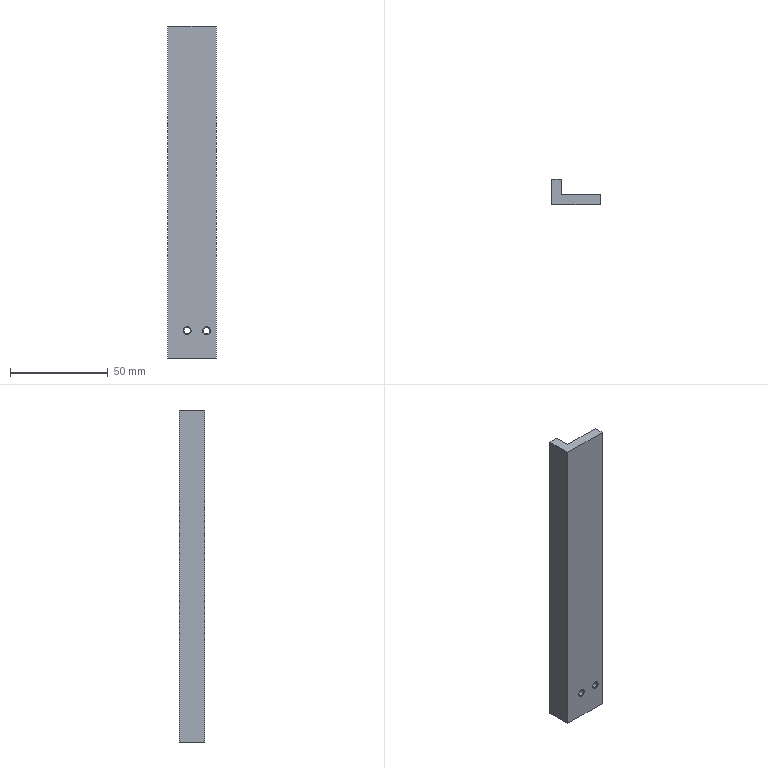Part | SolidWorks | features 3DProfileFeature 1, Extrusion 1, HoleWzd 1 | 1 solid | 16 faces | box 25 x 13 x 170 mm | volume 27963 mm3 | plane 8 | cone 4 | cylinder 4 | commonest cylinder face diameters 3.3 x4
STEP:
#1=CARTESIAN_POINT('',(10.,0.375,15.65));
#2=VERTEX_POINT('',#1);
#3=CARTESIAN_POINT('',(10.,0.375,12.35));
#4=VERTEX_POINT('',#3);
#5=CARTESIAN_POINT('',(10.,0.375,14.));
#6=DIRECTION('',(0.,-1.,0.));
#7=DIRECTION('',(0.,0.,-1.));
#8=AXIS2_PLACEMENT_3D('',#5,#6,#7);
#9=CIRCLE('',#8,1.65);
#10=EDGE_CURVE('',#2,#4,#9,.T.);
#11=ORIENTED_EDGE('',*,*,#10,.F.);
#12=CARTESIAN_POINT('',(10.,0.,16.025));
#13=VERTEX_POINT('',#12);
#14=CARTESIAN_POINT('',(10.,0.,16.025));
#15=DIRECTION('',(0.,-0.7071,0.7071));
#16=VECTOR('',#15,1000.);
#17=LINE('',#14,#16);
#18=EDGE_CURVE('',#2,#13,#17,.T.);
#19=ORIENTED_EDGE('',*,*,#18,.T.);
#20=CARTESIAN_POINT('',(10.,0.,11.975));
#21=VERTEX_POINT('',#20);
#22=CARTESIAN_POINT('',(10.,0.,14.));
#23=DIRECTION('',(0.,-1.,0.));
#24=DIRECTION('',(0.,0.,-1.));
#25=AXIS2_PLACEMENT_3D('',#22,#23,#24);
#26=CIRCLE('',#25,2.025);
#27=EDGE_CURVE('',#13,#21,#26,.T.);
#28=ORIENTED_EDGE('',*,*,#27,.T.);
#29=CARTESIAN_POINT('',(10.,0.,11.975));
#30=DIRECTION('',(0.,-0.7071,-0.7071));
#31=VECTOR('',#30,1000.);
#32=LINE('',#29,#31);
#33=EDGE_CURVE('',#4,#21,#32,.T.);
#34=ORIENTED_EDGE('',*,*,#33,.F.);
#35=EDGE_LOOP('',(#11,#19,#28,#34));
#36=FACE_OUTER_BOUND('',#35,.T.);
#37=CARTESIAN_POINT('',(10.,0.,14.));
#38=DIRECTION('',(0.,-1.,0.));
#39=DIRECTION('',(0.,0.,-1.));
#40=AXIS2_PLACEMENT_3D('',#37,#38,#39);
#41=CONICAL_SURFACE('',#40,2.025,0.7854);
#42=ADVANCED_FACE('',(#36),#41,.F.);
#43=CARTESIAN_POINT('',(10.,5.,15.65));
#44=VERTEX_POINT('',#43);
#45=CARTESIAN_POINT('',(10.,5.,12.35));
#46=VERTEX_POINT('',#45);
#47=CARTESIAN_POINT('',(10.,5.,14.));
#48=DIRECTION('',(0.,-1.,0.));
#49=DIRECTION('',(0.,0.,-1.));
#50=AXIS2_PLACEMENT_3D('',#47,#48,#49);
#51=CIRCLE('',#50,1.65);
#52=EDGE_CURVE('',#44,#46,#51,.T.);
#53=ORIENTED_EDGE('',*,*,#52,.F.);
#54=CARTESIAN_POINT('',(10.,0.,15.65));
#55=DIRECTION('',(0.,-1.,0.));
#56=VECTOR('',#55,1000.);
#57=LINE('',#54,#56);
#58=EDGE_CURVE('',#44,#2,#57,.T.);
#59=ORIENTED_EDGE('',*,*,#58,.T.);
#60=ORIENTED_EDGE('',*,*,#10,.T.);
#61=CARTESIAN_POINT('',(10.,0.,12.35));
#62=DIRECTION('',(0.,-1.,0.));
#63=VECTOR('',#62,1000.);
#64=LINE('',#61,#63);
#65=EDGE_CURVE('',#46,#4,#64,.T.);
#66=ORIENTED_EDGE('',*,*,#65,.F.);
#67=EDGE_LOOP('',(#53,#59,#60,#66));
#68=FACE_OUTER_BOUND('',#67,.T.);
#69=CARTESIAN_POINT('',(10.,0.,14.));
#70=DIRECTION('',(0.,-1.,0.));
#71=DIRECTION('',(0.,0.,-1.));
#72=AXIS2_PLACEMENT_3D('',#69,#70,#71);
#73=CYLINDRICAL_SURFACE('',#72,1.65);
#74=ADVANCED_FACE('',(#68),#73,.F.);
#75=CARTESIAN_POINT('',(20.,0.375,15.65));
#76=VERTEX_POINT('',#75);
#77=CARTESIAN_POINT('',(20.,0.375,12.35));
#78=VERTEX_POINT('',#77);
#79=CARTESIAN_POINT('',(20.,0.375,14.));
#80=DIRECTION('',(0.,-1.,0.));
#81=DIRECTION('',(0.,0.,-1.));
#82=AXIS2_PLACEMENT_3D('',#79,#80,#81);
#83=CIRCLE('',#82,1.65);
#84=EDGE_CURVE('',#76,#78,#83,.T.);
#85=ORIENTED_EDGE('',*,*,#84,.F.);
#86=CARTESIAN_POINT('',(20.,0.,16.025));
#87=VERTEX_POINT('',#86);
#88=CARTESIAN_POINT('',(20.,0.,16.025));
#89=DIRECTION('',(0.,-0.7071,0.7071));
#90=VECTOR('',#89,1000.);
#91=LINE('',#88,#90);
#92=EDGE_CURVE('',#76,#87,#91,.T.);
#93=ORIENTED_EDGE('',*,*,#92,.T.);
#94=CARTESIAN_POINT('',(20.,0.,11.975));
#95=VERTEX_POINT('',#94);
#96=CARTESIAN_POINT('',(20.,0.,14.));
#97=DIRECTION('',(0.,-1.,0.));
#98=DIRECTION('',(0.,0.,-1.));
#99=AXIS2_PLACEMENT_3D('',#96,#97,#98);
#100=CIRCLE('',#99,2.025);
#101=EDGE_CURVE('',#87,#95,#100,.T.);
#102=ORIENTED_EDGE('',*,*,#101,.T.);
#103=CARTESIAN_POINT('',(20.,0.,11.975));
#104=DIRECTION('',(0.,-0.7071,-0.7071));
#105=VECTOR('',#104,1000.);
#106=LINE('',#103,#105);
#107=EDGE_CURVE('',#78,#95,#106,.T.);
#108=ORIENTED_EDGE('',*,*,#107,.F.);
#109=EDGE_LOOP('',(#85,#93,#102,#108));
#110=FACE_OUTER_BOUND('',#109,.T.);
#111=CARTESIAN_POINT('',(20.,0.,14.));
#112=DIRECTION('',(0.,-1.,0.));
#113=DIRECTION('',(0.,0.,-1.));
#114=AXIS2_PLACEMENT_3D('',#111,#112,#113);
#115=CONICAL_SURFACE('',#114,2.025,0.7854);
#116=ADVANCED_FACE('',(#110),#115,.F.);
#117=CARTESIAN_POINT('',(20.,5.,15.65));
#118=VERTEX_POINT('',#117);
#119=CARTESIAN_POINT('',(20.,5.,12.35));
#120=VERTEX_POINT('',#119);
#121=CARTESIAN_POINT('',(20.,5.,14.));
#122=DIRECTION('',(0.,-1.,0.));
#123=DIRECTION('',(0.,0.,-1.));
#124=AXIS2_PLACEMENT_3D('',#121,#122,#123);
#125=CIRCLE('',#124,1.65);
#126=EDGE_CURVE('',#118,#120,#125,.T.);
#127=ORIENTED_EDGE('',*,*,#126,.F.);
#128=CARTESIAN_POINT('',(20.,0.,15.65));
#129=DIRECTION('',(0.,-1.,0.));
#130=VECTOR('',#129,1000.);
#131=LINE('',#128,#130);
#132=EDGE_CURVE('',#118,#76,#131,.T.);
#133=ORIENTED_EDGE('',*,*,#132,.T.);
#134=ORIENTED_EDGE('',*,*,#84,.T.);
#135=CARTESIAN_POINT('',(20.,0.,12.35));
#136=DIRECTION('',(0.,-1.,0.));
#137=VECTOR('',#136,1000.);
#138=LINE('',#135,#137);
#139=EDGE_CURVE('',#120,#78,#138,.T.);
#140=ORIENTED_EDGE('',*,*,#139,.F.);
#141=EDGE_LOOP('',(#127,#133,#134,#140));
#142=FACE_OUTER_BOUND('',#141,.T.);
#143=CARTESIAN_POINT('',(20.,0.,14.));
#144=DIRECTION('',(0.,-1.,0.));
#145=DIRECTION('',(0.,0.,-1.));
#146=AXIS2_PLACEMENT_3D('',#143,#144,#145);
#147=CYLINDRICAL_SURFACE('',#146,1.65);
#148=ADVANCED_FACE('',(#142),#147,.F.);
#149=CARTESIAN_POINT('',(10.,0.,14.));
#150=DIRECTION('',(0.,-1.,0.));
#151=DIRECTION('',(0.,0.,-1.));
#152=AXIS2_PLACEMENT_3D('',#149,#150,#151);
#153=CIRCLE('',#152,2.025);
#154=EDGE_CURVE('',#21,#13,#153,.T.);
#155=ORIENTED_EDGE('',*,*,#154,.F.);
#156=ORIENTED_EDGE('',*,*,#27,.F.);
#157=EDGE_LOOP('',(#155,#156));
#158=FACE_BOUND('',#157,.T.);
#159=CARTESIAN_POINT('',(20.,0.,14.));
#160=DIRECTION('',(0.,-1.,0.));
#161=DIRECTION('',(0.,0.,-1.));
#162=AXIS2_PLACEMENT_3D('',#159,#160,#161);
#163=CIRCLE('',#162,2.025);
#164=EDGE_CURVE('',#95,#87,#163,.T.);
#165=ORIENTED_EDGE('',*,*,#164,.F.);
#166=ORIENTED_EDGE('',*,*,#101,.F.);
#167=EDGE_LOOP('',(#165,#166));
#168=FACE_BOUND('',#167,.T.);
#169=CARTESIAN_POINT('',(0.,0.,0.));
#170=VERTEX_POINT('',#169);
#171=CARTESIAN_POINT('',(25.,0.,0.));
#172=VERTEX_POINT('',#171);
#173=CARTESIAN_POINT('',(25.,0.,0.));
#174=DIRECTION('',(1.,0.,0.));
#175=VECTOR('',#174,1000.);
#176=LINE('',#173,#175);
#177=EDGE_CURVE('',#170,#172,#176,.T.);
#178=ORIENTED_EDGE('',*,*,#177,.T.);
#179=CARTESIAN_POINT('',(25.,0.,170.));
#180=VERTEX_POINT('',#179);
#181=CARTESIAN_POINT('',(25.,0.,170.));
#182=DIRECTION('',(0.,0.,-1.));
#183=VECTOR('',#182,1000.);
#184=LINE('',#181,#183);
#185=EDGE_CURVE('',#180,#172,#184,.T.);
#186=ORIENTED_EDGE('',*,*,#185,.F.);
#187=CARTESIAN_POINT('',(0.,0.,170.));
#188=VERTEX_POINT('',#187);
#189=CARTESIAN_POINT('',(25.,0.,170.));
#190=DIRECTION('',(1.,0.,0.));
#191=VECTOR('',#190,1000.);
#192=LINE('',#189,#191);
#193=EDGE_CURVE('',#188,#180,#192,.T.);
#194=ORIENTED_EDGE('',*,*,#193,.F.);
#195=CARTESIAN_POINT('',(0.,0.,170.));
#196=DIRECTION('',(0.,0.,-1.));
#197=VECTOR('',#196,1000.);
#198=LINE('',#195,#197);
#199=EDGE_CURVE('',#188,#170,#198,.T.);
#200=ORIENTED_EDGE('',*,*,#199,.T.);
#201=EDGE_LOOP('',(#178,#186,#194,#200));
#202=FACE_OUTER_BOUND('',#201,.T.);
#203=CARTESIAN_POINT('',(25.,0.,170.));
#204=DIRECTION('',(0.,1.,0.));
#205=DIRECTION('',(-1.,0.,0.));
#206=AXIS2_PLACEMENT_3D('',#203,#204,#205);
#207=PLANE('',#206);
#208=ADVANCED_FACE('',(#158,#168,#202),#207,.F.);
#209=CARTESIAN_POINT('',(25.,5.,0.));
#210=VERTEX_POINT('',#209);
#211=CARTESIAN_POINT('',(25.,5.,0.));
#212=DIRECTION('',(0.,1.,0.));
#213=VECTOR('',#212,1000.);
#214=LINE('',#211,#213);
#215=EDGE_CURVE('',#172,#210,#214,.T.);
#216=ORIENTED_EDGE('',*,*,#215,.T.);
#217=CARTESIAN_POINT('',(25.,5.,170.));
#218=VERTEX_POINT('',#217);
#219=CARTESIAN_POINT('',(25.,5.,170.));
#220=DIRECTION('',(0.,0.,-1.));
#221=VECTOR('',#220,1000.);
#222=LINE('',#219,#221);
#223=EDGE_CURVE('',#218,#210,#222,.T.);
#224=ORIENTED_EDGE('',*,*,#223,.F.);
#225=CARTESIAN_POINT('',(25.,5.,170.));
#226=DIRECTION('',(0.,1.,0.));
#227=VECTOR('',#226,1000.);
#228=LINE('',#225,#227);
#229=EDGE_CURVE('',#180,#218,#228,.T.);
#230=ORIENTED_EDGE('',*,*,#229,.F.);
#231=ORIENTED_EDGE('',*,*,#185,.T.);
#232=EDGE_LOOP('',(#216,#224,#230,#231));
#233=FACE_OUTER_BOUND('',#232,.T.);
#234=CARTESIAN_POINT('',(25.,5.,170.));
#235=DIRECTION('',(-1.,0.,0.));
#236=DIRECTION('',(0.,0.,1.));
#237=AXIS2_PLACEMENT_3D('',#234,#235,#236);
#238=PLANE('',#237);
#239=ADVANCED_FACE('',(#233),#238,.F.);
#240=CARTESIAN_POINT('',(10.,5.,14.));
#241=DIRECTION('',(0.,-1.,0.));
#242=DIRECTION('',(0.,0.,-1.));
#243=AXIS2_PLACEMENT_3D('',#240,#241,#242);
#244=CIRCLE('',#243,1.65);
#245=EDGE_CURVE('',#46,#44,#244,.T.);
#246=ORIENTED_EDGE('',*,*,#245,.T.);
#247=ORIENTED_EDGE('',*,*,#52,.T.);
#248=EDGE_LOOP('',(#246,#247));
#249=FACE_BOUND('',#248,.T.);
#250=CARTESIAN_POINT('',(20.,5.,14.));
#251=DIRECTION('',(0.,-1.,0.));
#252=DIRECTION('',(0.,0.,-1.));
#253=AXIS2_PLACEMENT_3D('',#250,#251,#252);
#254=CIRCLE('',#253,1.65);
#255=EDGE_CURVE('',#120,#118,#254,.T.);
#256=ORIENTED_EDGE('',*,*,#255,.T.);
#257=ORIENTED_EDGE('',*,*,#126,.T.);
#258=EDGE_LOOP('',(#256,#257));
#259=FACE_BOUND('',#258,.T.);
#260=CARTESIAN_POINT('',(5.,5.,0.));
#261=VERTEX_POINT('',#260);
#262=CARTESIAN_POINT('',(5.,5.,0.));
#263=DIRECTION('',(-1.,0.,0.));
#264=VECTOR('',#263,1000.);
#265=LINE('',#262,#264);
#266=EDGE_CURVE('',#210,#261,#265,.T.);
#267=ORIENTED_EDGE('',*,*,#266,.T.);
#268=CARTESIAN_POINT('',(5.,5.,170.));
#269=VERTEX_POINT('',#268);
#270=CARTESIAN_POINT('',(5.,5.,170.));
#271=DIRECTION('',(0.,0.,-1.));
#272=VECTOR('',#271,1000.);
#273=LINE('',#270,#272);
#274=EDGE_CURVE('',#269,#261,#273,.T.);
#275=ORIENTED_EDGE('',*,*,#274,.F.);
#276=CARTESIAN_POINT('',(5.,5.,170.));
#277=DIRECTION('',(-1.,0.,0.));
#278=VECTOR('',#277,1000.);
#279=LINE('',#276,#278);
#280=EDGE_CURVE('',#218,#269,#279,.T.);
#281=ORIENTED_EDGE('',*,*,#280,.F.);
#282=ORIENTED_EDGE('',*,*,#223,.T.);
#283=EDGE_LOOP('',(#267,#275,#281,#282));
#284=FACE_OUTER_BOUND('',#283,.T.);
#285=CARTESIAN_POINT('',(5.,5.,170.));
#286=DIRECTION('',(0.,-1.,0.));
#287=DIRECTION('',(0.,0.,-1.));
#288=AXIS2_PLACEMENT_3D('',#285,#286,#287);
#289=PLANE('',#288);
#290=ADVANCED_FACE('',(#249,#259,#284),#289,.F.);
#291=CARTESIAN_POINT('',(5.,13.,0.));
#292=VERTEX_POINT('',#291);
#293=CARTESIAN_POINT('',(5.,13.,0.));
#294=DIRECTION('',(0.,1.,0.));
#295=VECTOR('',#294,1000.);
#296=LINE('',#293,#295);
#297=EDGE_CURVE('',#261,#292,#296,.T.);
#298=ORIENTED_EDGE('',*,*,#297,.T.);
#299=CARTESIAN_POINT('',(5.,13.,170.));
#300=VERTEX_POINT('',#299);
#301=CARTESIAN_POINT('',(5.,13.,170.));
#302=DIRECTION('',(0.,0.,-1.));
#303=VECTOR('',#302,1000.);
#304=LINE('',#301,#303);
#305=EDGE_CURVE('',#300,#292,#304,.T.);
#306=ORIENTED_EDGE('',*,*,#305,.F.);
#307=CARTESIAN_POINT('',(5.,13.,170.));
#308=DIRECTION('',(0.,1.,0.));
#309=VECTOR('',#308,1000.);
#310=LINE('',#307,#309);
#311=EDGE_CURVE('',#269,#300,#310,.T.);
#312=ORIENTED_EDGE('',*,*,#311,.F.);
#313=ORIENTED_EDGE('',*,*,#274,.T.);
#314=EDGE_LOOP('',(#298,#306,#312,#313));
#315=FACE_OUTER_BOUND('',#314,.T.);
#316=CARTESIAN_POINT('',(5.,13.,170.));
#317=DIRECTION('',(-1.,0.,0.));
#318=DIRECTION('',(0.,-1.,0.));
#319=AXIS2_PLACEMENT_3D('',#316,#317,#318);
#320=PLANE('',#319);
#321=ADVANCED_FACE('',(#315),#320,.F.);
#322=CARTESIAN_POINT('',(0.,13.,0.));
#323=VERTEX_POINT('',#322);
#324=CARTESIAN_POINT('',(0.,13.,0.));
#325=DIRECTION('',(-1.,0.,0.));
#326=VECTOR('',#325,1000.);
#327=LINE('',#324,#326);
#328=EDGE_CURVE('',#292,#323,#327,.T.);
#329=ORIENTED_EDGE('',*,*,#328,.T.);
#330=CARTESIAN_POINT('',(0.,13.,170.));
#331=VERTEX_POINT('',#330);
#332=CARTESIAN_POINT('',(0.,13.,170.));
#333=DIRECTION('',(0.,0.,-1.));
#334=VECTOR('',#333,1000.);
#335=LINE('',#332,#334);
#336=EDGE_CURVE('',#331,#323,#335,.T.);
#337=ORIENTED_EDGE('',*,*,#336,.F.);
#338=CARTESIAN_POINT('',(0.,13.,170.));
#339=DIRECTION('',(-1.,0.,0.));
#340=VECTOR('',#339,1000.);
#341=LINE('',#338,#340);
#342=EDGE_CURVE('',#300,#331,#341,.T.);
#343=ORIENTED_EDGE('',*,*,#342,.F.);
#344=ORIENTED_EDGE('',*,*,#305,.T.);
#345=EDGE_LOOP('',(#329,#337,#343,#344));
#346=FACE_OUTER_BOUND('',#345,.T.);
#347=CARTESIAN_POINT('',(0.,13.,170.));
#348=DIRECTION('',(0.,-1.,0.));
#349=DIRECTION('',(0.,0.,-1.));
#350=AXIS2_PLACEMENT_3D('',#347,#348,#349);
#351=PLANE('',#350);
#352=ADVANCED_FACE('',(#346),#351,.F.);
#353=CARTESIAN_POINT('',(0.,0.,0.));
#354=DIRECTION('',(0.,-1.,0.));
#355=VECTOR('',#354,1000.);
#356=LINE('',#353,#355);
#357=EDGE_CURVE('',#323,#170,#356,.T.);
#358=ORIENTED_EDGE('',*,*,#357,.T.);
#359=ORIENTED_EDGE('',*,*,#199,.F.);
#360=CARTESIAN_POINT('',(0.,0.,170.));
#361=DIRECTION('',(0.,-1.,0.));
#362=VECTOR('',#361,1000.);
#363=LINE('',#360,#362);
#364=EDGE_CURVE('',#331,#188,#363,.T.);
#365=ORIENTED_EDGE('',*,*,#364,.F.);
#366=ORIENTED_EDGE('',*,*,#336,.T.);
#367=EDGE_LOOP('',(#358,#359,#365,#366));
#368=FACE_OUTER_BOUND('',#367,.T.);
#369=CARTESIAN_POINT('',(0.,0.,170.));
#370=DIRECTION('',(1.,0.,0.));
#371=DIRECTION('',(0.,1.,0.));
#372=AXIS2_PLACEMENT_3D('',#369,#370,#371);
#373=PLANE('',#372);
#374=ADVANCED_FACE('',(#368),#373,.F.);
#375=ORIENTED_EDGE('',*,*,#193,.T.);
#376=ORIENTED_EDGE('',*,*,#229,.T.);
#377=ORIENTED_EDGE('',*,*,#280,.T.);
#378=ORIENTED_EDGE('',*,*,#311,.T.);
#379=ORIENTED_EDGE('',*,*,#342,.T.);
#380=ORIENTED_EDGE('',*,*,#364,.T.);
#381=EDGE_LOOP('',(#375,#376,#377,#378,#379,#380));
#382=FACE_OUTER_BOUND('',#381,.T.);
#383=CARTESIAN_POINT('',(0.,0.,170.));
#384=DIRECTION('',(0.,0.,-1.));
#385=DIRECTION('',(-1.,0.,0.));
#386=AXIS2_PLACEMENT_3D('',#383,#384,#385);
#387=PLANE('',#386);
#388=ADVANCED_FACE('',(#382),#387,.F.);
#389=ORIENTED_EDGE('',*,*,#177,.F.);
#390=ORIENTED_EDGE('',*,*,#357,.F.);
#391=ORIENTED_EDGE('',*,*,#328,.F.);
#392=ORIENTED_EDGE('',*,*,#297,.F.);
#393=ORIENTED_EDGE('',*,*,#266,.F.);
#394=ORIENTED_EDGE('',*,*,#215,.F.);
#395=EDGE_LOOP('',(#389,#390,#391,#392,#393,#394));
#396=FACE_OUTER_BOUND('',#395,.T.);
#397=CARTESIAN_POINT('',(0.,0.,0.));
#398=DIRECTION('',(0.,0.,-1.));
#399=DIRECTION('',(-1.,0.,0.));
#400=AXIS2_PLACEMENT_3D('',#397,#398,#399);
#401=PLANE('',#400);
#402=ADVANCED_FACE('',(#396),#401,.T.);
#403=ORIENTED_EDGE('',*,*,#132,.F.);
#404=ORIENTED_EDGE('',*,*,#255,.F.);
#405=ORIENTED_EDGE('',*,*,#139,.T.);
#406=CARTESIAN_POINT('',(20.,0.375,14.));
#407=DIRECTION('',(0.,-1.,0.));
#408=DIRECTION('',(0.,0.,-1.));
#409=AXIS2_PLACEMENT_3D('',#406,#407,#408);
#410=CIRCLE('',#409,1.65);
#411=EDGE_CURVE('',#78,#76,#410,.T.);
#412=ORIENTED_EDGE('',*,*,#411,.T.);
#413=EDGE_LOOP('',(#403,#404,#405,#412));
#414=FACE_OUTER_BOUND('',#413,.T.);
#415=CARTESIAN_POINT('',(20.,0.,14.));
#416=DIRECTION('',(0.,-1.,0.));
#417=DIRECTION('',(0.,0.,-1.));
#418=AXIS2_PLACEMENT_3D('',#415,#416,#417);
#419=CYLINDRICAL_SURFACE('',#418,1.65);
#420=ADVANCED_FACE('',(#414),#419,.F.);
#421=ORIENTED_EDGE('',*,*,#92,.F.);
#422=ORIENTED_EDGE('',*,*,#411,.F.);
#423=ORIENTED_EDGE('',*,*,#107,.T.);
#424=ORIENTED_EDGE('',*,*,#164,.T.);
#425=EDGE_LOOP('',(#421,#422,#423,#424));
#426=FACE_OUTER_BOUND('',#425,.T.);
#427=CARTESIAN_POINT('',(20.,0.,14.));
#428=DIRECTION('',(0.,-1.,0.));
#429=DIRECTION('',(0.,0.,-1.));
#430=AXIS2_PLACEMENT_3D('',#427,#428,#429);
#431=CONICAL_SURFACE('',#430,2.025,0.7854);
#432=ADVANCED_FACE('',(#426),#431,.F.);
#433=ORIENTED_EDGE('',*,*,#58,.F.);
#434=ORIENTED_EDGE('',*,*,#245,.F.);
#435=ORIENTED_EDGE('',*,*,#65,.T.);
#436=CARTESIAN_POINT('',(10.,0.375,14.));
#437=DIRECTION('',(0.,-1.,0.));
#438=DIRECTION('',(0.,0.,-1.));
#439=AXIS2_PLACEMENT_3D('',#436,#437,#438);
#440=CIRCLE('',#439,1.65);
#441=EDGE_CURVE('',#4,#2,#440,.T.);
#442=ORIENTED_EDGE('',*,*,#441,.T.);
#443=EDGE_LOOP('',(#433,#434,#435,#442));
#444=FACE_OUTER_BOUND('',#443,.T.);
#445=CARTESIAN_POINT('',(10.,0.,14.));
#446=DIRECTION('',(0.,-1.,0.));
#447=DIRECTION('',(0.,0.,-1.));
#448=AXIS2_PLACEMENT_3D('',#445,#446,#447);
#449=CYLINDRICAL_SURFACE('',#448,1.65);
#450=ADVANCED_FACE('',(#444),#449,.F.);
#451=ORIENTED_EDGE('',*,*,#18,.F.);
#452=ORIENTED_EDGE('',*,*,#441,.F.);
#453=ORIENTED_EDGE('',*,*,#33,.T.);
#454=ORIENTED_EDGE('',*,*,#154,.T.);
#455=EDGE_LOOP('',(#451,#452,#453,#454));
#456=FACE_OUTER_BOUND('',#455,.T.);
#457=CARTESIAN_POINT('',(10.,0.,14.));
#458=DIRECTION('',(0.,-1.,0.));
#459=DIRECTION('',(0.,0.,-1.));
#460=AXIS2_PLACEMENT_3D('',#457,#458,#459);
#461=CONICAL_SURFACE('',#460,2.025,0.7854);
#462=ADVANCED_FACE('',(#456),#461,.F.);
#463=CLOSED_SHELL('',(#42,#74,#116,#148,#208,#239,#290,#321,#352,#374,#388,#402,#420,#432,#450,#462));
#464=MANIFOLD_SOLID_BREP('',#463);
#465=CARTESIAN_POINT('',(0.,0.,0.));
#466=DIRECTION('',(0.,0.,1.));
#467=DIRECTION('',(1.,0.,0.));
#468=AXIS2_PLACEMENT_3D('',#465,#466,#467);
#469=(LENGTH_UNIT()NAMED_UNIT(*)SI_UNIT(.MILLI.,.METRE.));
#470=UNCERTAINTY_MEASURE_WITH_UNIT(LENGTH_MEASURE(0.00001),#469,'','');
#471=(NAMED_UNIT(*)PLANE_ANGLE_UNIT()SI_UNIT($,.RADIAN.));
#472=(NAMED_UNIT(*)SI_UNIT($,.STERADIAN.)SOLID_ANGLE_UNIT());
#473=(GEOMETRIC_REPRESENTATION_CONTEXT(3)GLOBAL_UNCERTAINTY_ASSIGNED_CONTEXT((#470))GLOBAL_UNIT_ASSIGNED_CONTEXT((#469,#471,#472))REPRESENTATION_CONTEXT('',''));
#474=ADVANCED_BREP_SHAPE_REPRESENTATION('',(#464,#468),#473);